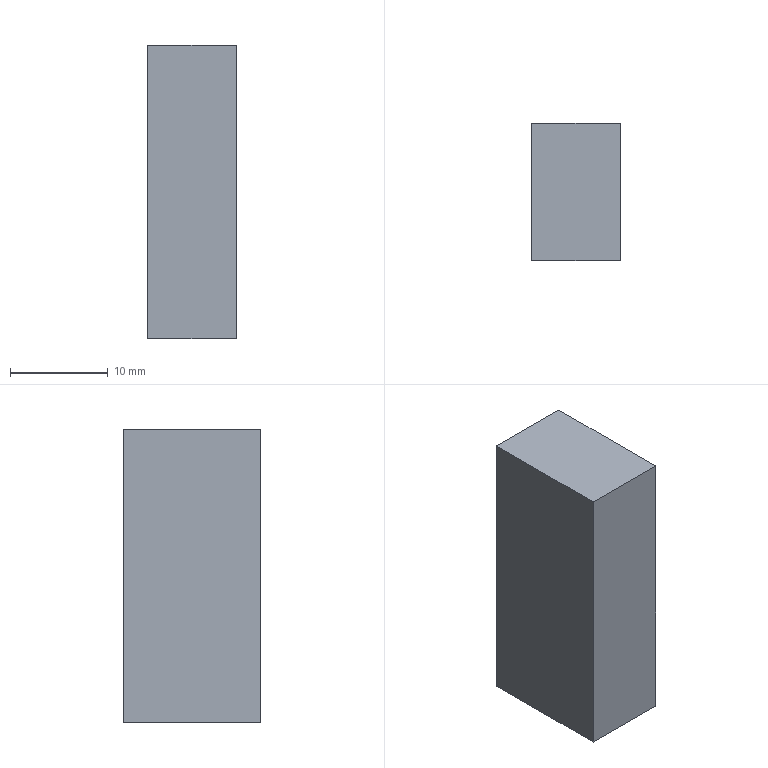Part | SolidWorks | features Extrusion 1 | 1 solid | 6 faces | box 9 x 14 x 30 mm | volume 3780 mm3 | plane 6
STEP:
#1=CARTESIAN_POINT('',(4.5,0.,15.));
#2=VERTEX_POINT('',#1);
#3=CARTESIAN_POINT('',(4.5,0.,-15.));
#4=VERTEX_POINT('',#3);
#5=CARTESIAN_POINT('',(4.5,0.,-15.));
#6=DIRECTION('',(0.,0.,-1.));
#7=VECTOR('',#6,1000.);
#8=LINE('',#5,#7);
#9=EDGE_CURVE('',#2,#4,#8,.T.);
#10=ORIENTED_EDGE('',*,*,#9,.T.);
#11=CARTESIAN_POINT('',(4.5,14.,-15.));
#12=VERTEX_POINT('',#11);
#13=CARTESIAN_POINT('',(4.5,14.,-15.));
#14=DIRECTION('',(0.,-1.,0.));
#15=VECTOR('',#14,1000.);
#16=LINE('',#13,#15);
#17=EDGE_CURVE('',#12,#4,#16,.T.);
#18=ORIENTED_EDGE('',*,*,#17,.F.);
#19=CARTESIAN_POINT('',(4.5,14.,15.));
#20=VERTEX_POINT('',#19);
#21=CARTESIAN_POINT('',(4.5,14.,-15.));
#22=DIRECTION('',(0.,0.,-1.));
#23=VECTOR('',#22,1000.);
#24=LINE('',#21,#23);
#25=EDGE_CURVE('',#20,#12,#24,.T.);
#26=ORIENTED_EDGE('',*,*,#25,.F.);
#27=CARTESIAN_POINT('',(4.5,14.,15.));
#28=DIRECTION('',(0.,-1.,0.));
#29=VECTOR('',#28,1000.);
#30=LINE('',#27,#29);
#31=EDGE_CURVE('',#20,#2,#30,.T.);
#32=ORIENTED_EDGE('',*,*,#31,.T.);
#33=EDGE_LOOP('',(#10,#18,#26,#32));
#34=FACE_OUTER_BOUND('',#33,.T.);
#35=CARTESIAN_POINT('',(4.5,14.,-15.));
#36=DIRECTION('',(-1.,0.,0.));
#37=DIRECTION('',(0.,0.,1.));
#38=AXIS2_PLACEMENT_3D('',#35,#36,#37);
#39=PLANE('',#38);
#40=ADVANCED_FACE('',(#34),#39,.F.);
#41=CARTESIAN_POINT('',(-4.5,0.,-15.));
#42=VERTEX_POINT('',#41);
#43=CARTESIAN_POINT('',(-4.5,0.,-15.));
#44=DIRECTION('',(-1.,0.,0.));
#45=VECTOR('',#44,1000.);
#46=LINE('',#43,#45);
#47=EDGE_CURVE('',#4,#42,#46,.T.);
#48=ORIENTED_EDGE('',*,*,#47,.T.);
#49=CARTESIAN_POINT('',(-4.5,14.,-15.));
#50=VERTEX_POINT('',#49);
#51=CARTESIAN_POINT('',(-4.5,14.,-15.));
#52=DIRECTION('',(0.,-1.,0.));
#53=VECTOR('',#52,1000.);
#54=LINE('',#51,#53);
#55=EDGE_CURVE('',#50,#42,#54,.T.);
#56=ORIENTED_EDGE('',*,*,#55,.F.);
#57=CARTESIAN_POINT('',(-4.5,14.,-15.));
#58=DIRECTION('',(-1.,0.,0.));
#59=VECTOR('',#58,1000.);
#60=LINE('',#57,#59);
#61=EDGE_CURVE('',#12,#50,#60,.T.);
#62=ORIENTED_EDGE('',*,*,#61,.F.);
#63=ORIENTED_EDGE('',*,*,#17,.T.);
#64=EDGE_LOOP('',(#48,#56,#62,#63));
#65=FACE_OUTER_BOUND('',#64,.T.);
#66=CARTESIAN_POINT('',(-4.5,14.,-15.));
#67=DIRECTION('',(0.,0.,1.));
#68=DIRECTION('',(1.,0.,0.));
#69=AXIS2_PLACEMENT_3D('',#66,#67,#68);
#70=PLANE('',#69);
#71=ADVANCED_FACE('',(#65),#70,.F.);
#72=CARTESIAN_POINT('',(-4.5,0.,15.));
#73=VERTEX_POINT('',#72);
#74=CARTESIAN_POINT('',(-4.5,0.,-15.));
#75=DIRECTION('',(0.,0.,1.));
#76=VECTOR('',#75,1000.);
#77=LINE('',#74,#76);
#78=EDGE_CURVE('',#42,#73,#77,.T.);
#79=ORIENTED_EDGE('',*,*,#78,.T.);
#80=CARTESIAN_POINT('',(-4.5,14.,15.));
#81=VERTEX_POINT('',#80);
#82=CARTESIAN_POINT('',(-4.5,14.,15.));
#83=DIRECTION('',(0.,-1.,0.));
#84=VECTOR('',#83,1000.);
#85=LINE('',#82,#84);
#86=EDGE_CURVE('',#81,#73,#85,.T.);
#87=ORIENTED_EDGE('',*,*,#86,.F.);
#88=CARTESIAN_POINT('',(-4.5,14.,-15.));
#89=DIRECTION('',(0.,0.,1.));
#90=VECTOR('',#89,1000.);
#91=LINE('',#88,#90);
#92=EDGE_CURVE('',#50,#81,#91,.T.);
#93=ORIENTED_EDGE('',*,*,#92,.F.);
#94=ORIENTED_EDGE('',*,*,#55,.T.);
#95=EDGE_LOOP('',(#79,#87,#93,#94));
#96=FACE_OUTER_BOUND('',#95,.T.);
#97=CARTESIAN_POINT('',(-4.5,14.,-15.));
#98=DIRECTION('',(1.,0.,0.));
#99=DIRECTION('',(0.,0.,-1.));
#100=AXIS2_PLACEMENT_3D('',#97,#98,#99);
#101=PLANE('',#100);
#102=ADVANCED_FACE('',(#96),#101,.F.);
#103=CARTESIAN_POINT('',(-4.5,0.,15.));
#104=DIRECTION('',(1.,0.,0.));
#105=VECTOR('',#104,1000.);
#106=LINE('',#103,#105);
#107=EDGE_CURVE('',#73,#2,#106,.T.);
#108=ORIENTED_EDGE('',*,*,#107,.T.);
#109=ORIENTED_EDGE('',*,*,#31,.F.);
#110=CARTESIAN_POINT('',(-4.5,14.,15.));
#111=DIRECTION('',(1.,0.,0.));
#112=VECTOR('',#111,1000.);
#113=LINE('',#110,#112);
#114=EDGE_CURVE('',#81,#20,#113,.T.);
#115=ORIENTED_EDGE('',*,*,#114,.F.);
#116=ORIENTED_EDGE('',*,*,#86,.T.);
#117=EDGE_LOOP('',(#108,#109,#115,#116));
#118=FACE_OUTER_BOUND('',#117,.T.);
#119=CARTESIAN_POINT('',(-4.5,14.,15.));
#120=DIRECTION('',(0.,0.,-1.));
#121=DIRECTION('',(-1.,0.,0.));
#122=AXIS2_PLACEMENT_3D('',#119,#120,#121);
#123=PLANE('',#122);
#124=ADVANCED_FACE('',(#118),#123,.F.);
#125=ORIENTED_EDGE('',*,*,#25,.T.);
#126=ORIENTED_EDGE('',*,*,#61,.T.);
#127=ORIENTED_EDGE('',*,*,#92,.T.);
#128=ORIENTED_EDGE('',*,*,#114,.T.);
#129=EDGE_LOOP('',(#125,#126,#127,#128));
#130=FACE_OUTER_BOUND('',#129,.T.);
#131=CARTESIAN_POINT('',(0.,14.,0.));
#132=DIRECTION('',(0.,1.,0.));
#133=DIRECTION('',(0.,0.,1.));
#134=AXIS2_PLACEMENT_3D('',#131,#132,#133);
#135=PLANE('',#134);
#136=ADVANCED_FACE('',(#130),#135,.T.);
#137=ORIENTED_EDGE('',*,*,#9,.F.);
#138=ORIENTED_EDGE('',*,*,#107,.F.);
#139=ORIENTED_EDGE('',*,*,#78,.F.);
#140=ORIENTED_EDGE('',*,*,#47,.F.);
#141=EDGE_LOOP('',(#137,#138,#139,#140));
#142=FACE_OUTER_BOUND('',#141,.T.);
#143=CARTESIAN_POINT('',(0.,0.,0.));
#144=DIRECTION('',(0.,1.,0.));
#145=DIRECTION('',(0.,0.,1.));
#146=AXIS2_PLACEMENT_3D('',#143,#144,#145);
#147=PLANE('',#146);
#148=ADVANCED_FACE('',(#142),#147,.F.);
#149=CLOSED_SHELL('',(#40,#71,#102,#124,#136,#148));
#150=MANIFOLD_SOLID_BREP('',#149);
#151=CARTESIAN_POINT('',(0.,0.,0.));
#152=DIRECTION('',(0.,0.,1.));
#153=DIRECTION('',(1.,0.,0.));
#154=AXIS2_PLACEMENT_3D('',#151,#152,#153);
#155=(LENGTH_UNIT()NAMED_UNIT(*)SI_UNIT(.MILLI.,.METRE.));
#156=UNCERTAINTY_MEASURE_WITH_UNIT(LENGTH_MEASURE(0.00001),#155,'','');
#157=(NAMED_UNIT(*)PLANE_ANGLE_UNIT()SI_UNIT($,.RADIAN.));
#158=(NAMED_UNIT(*)SI_UNIT($,.STERADIAN.)SOLID_ANGLE_UNIT());
#159=(GEOMETRIC_REPRESENTATION_CONTEXT(3)GLOBAL_UNCERTAINTY_ASSIGNED_CONTEXT((#156))GLOBAL_UNIT_ASSIGNED_CONTEXT((#155,#157,#158))REPRESENTATION_CONTEXT('',''));
#160=ADVANCED_BREP_SHAPE_REPRESENTATION('',(#150,#154),#159);